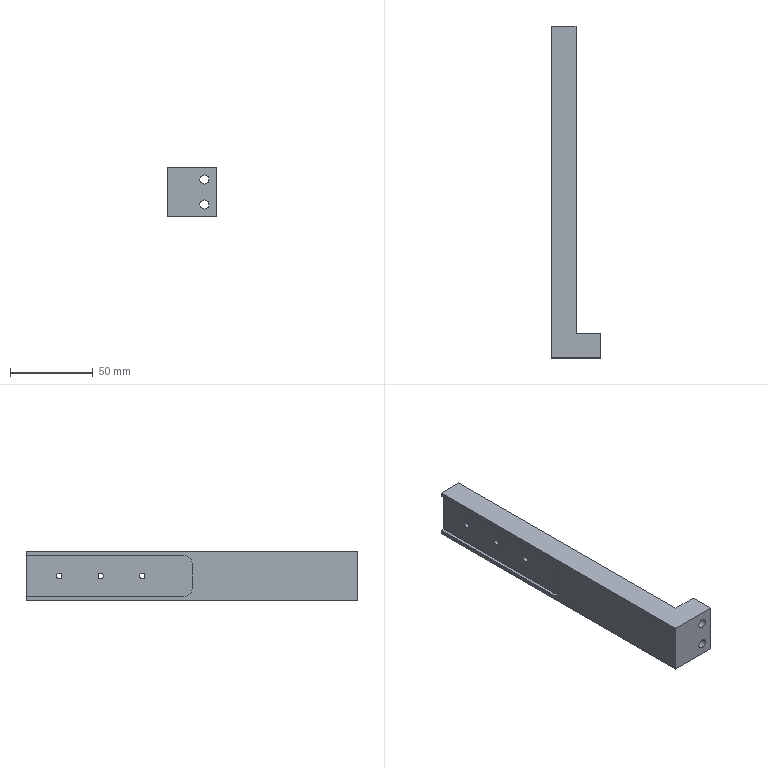Part | NX | 1 solid | 19 faces | box 30 x 200 x 30 mm | volume 90725 mm3 | plane 12 | cylinder 7 | commonest cylinder face diameters 3.3 x3 5.5 x2 10 x2
STEP:
#1=CARTESIAN_POINT('',(2.,105.,2.5));
#2=VERTEX_POINT('',#1);
#3=CARTESIAN_POINT('',(2.,100.,7.5));
#4=VERTEX_POINT('',#3);
#5=CARTESIAN_POINT('',(2.,105.,7.5));
#6=DIRECTION('',(-1.,0.,0.));
#7=DIRECTION('',(0.,1.,0.));
#8=AXIS2_PLACEMENT_3D('',#5,#6,#7);
#9=CIRCLE('',#8,5.);
#10=EDGE_CURVE('',#2,#4,#9,.T.);
#11=ORIENTED_EDGE('',*,*,#10,.F.);
#12=CARTESIAN_POINT('',(0.,105.,2.5));
#13=VERTEX_POINT('',#12);
#14=CARTESIAN_POINT('',(2.,105.,2.5));
#15=DIRECTION('',(1.,0.,0.));
#16=VECTOR('',#15,1000.);
#17=LINE('',#14,#16);
#18=EDGE_CURVE('',#13,#2,#17,.T.);
#19=ORIENTED_EDGE('',*,*,#18,.F.);
#20=CARTESIAN_POINT('',(0.,100.,7.5));
#21=VERTEX_POINT('',#20);
#22=CARTESIAN_POINT('',(0.,105.,7.5));
#23=DIRECTION('',(1.,0.,0.));
#24=DIRECTION('',(0.,1.,0.));
#25=AXIS2_PLACEMENT_3D('',#22,#23,#24);
#26=CIRCLE('',#25,5.);
#27=EDGE_CURVE('',#21,#13,#26,.T.);
#28=ORIENTED_EDGE('',*,*,#27,.F.);
#29=CARTESIAN_POINT('',(0.,100.,7.5));
#30=DIRECTION('',(-1.,0.,0.));
#31=VECTOR('',#30,1000.);
#32=LINE('',#29,#31);
#33=EDGE_CURVE('',#4,#21,#32,.T.);
#34=ORIENTED_EDGE('',*,*,#33,.F.);
#35=EDGE_LOOP('',(#11,#19,#28,#34));
#36=FACE_BOUND('',#35,.T.);
#37=CARTESIAN_POINT('',(2.,105.,7.5));
#38=DIRECTION('',(1.,0.,0.));
#39=DIRECTION('',(0.,1.,0.));
#40=AXIS2_PLACEMENT_3D('',#37,#38,#39);
#41=CYLINDRICAL_SURFACE('',#40,5.);
#42=ADVANCED_FACE('',(#36),#41,.F.);
#43=CARTESIAN_POINT('',(2.,100.,22.5));
#44=VERTEX_POINT('',#43);
#45=CARTESIAN_POINT('',(2.,105.,27.5));
#46=VERTEX_POINT('',#45);
#47=CARTESIAN_POINT('',(2.,105.,22.5));
#48=DIRECTION('',(-1.,0.,0.));
#49=DIRECTION('',(0.,1.,0.));
#50=AXIS2_PLACEMENT_3D('',#47,#48,#49);
#51=CIRCLE('',#50,5.);
#52=EDGE_CURVE('',#44,#46,#51,.T.);
#53=ORIENTED_EDGE('',*,*,#52,.F.);
#54=CARTESIAN_POINT('',(0.,100.,22.5));
#55=VERTEX_POINT('',#54);
#56=CARTESIAN_POINT('',(2.,100.,22.5));
#57=DIRECTION('',(1.,0.,0.));
#58=VECTOR('',#57,1000.);
#59=LINE('',#56,#58);
#60=EDGE_CURVE('',#55,#44,#59,.T.);
#61=ORIENTED_EDGE('',*,*,#60,.F.);
#62=CARTESIAN_POINT('',(0.,105.,27.5));
#63=VERTEX_POINT('',#62);
#64=CARTESIAN_POINT('',(0.,105.,22.5));
#65=DIRECTION('',(1.,0.,0.));
#66=DIRECTION('',(0.,1.,0.));
#67=AXIS2_PLACEMENT_3D('',#64,#65,#66);
#68=CIRCLE('',#67,5.);
#69=EDGE_CURVE('',#63,#55,#68,.T.);
#70=ORIENTED_EDGE('',*,*,#69,.F.);
#71=CARTESIAN_POINT('',(0.,105.,27.5));
#72=DIRECTION('',(-1.,0.,0.));
#73=VECTOR('',#72,1000.);
#74=LINE('',#71,#73);
#75=EDGE_CURVE('',#46,#63,#74,.T.);
#76=ORIENTED_EDGE('',*,*,#75,.F.);
#77=EDGE_LOOP('',(#53,#61,#70,#76));
#78=FACE_BOUND('',#77,.T.);
#79=CARTESIAN_POINT('',(2.,105.,22.5));
#80=DIRECTION('',(1.,0.,0.));
#81=DIRECTION('',(0.,1.,0.));
#82=AXIS2_PLACEMENT_3D('',#79,#80,#81);
#83=CYLINDRICAL_SURFACE('',#82,5.);
#84=ADVANCED_FACE('',(#78),#83,.F.);
#85=CARTESIAN_POINT('',(2.,100.,27.5));
#86=DIRECTION('',(0.,0.,1.));
#87=VECTOR('',#86,1000.);
#88=LINE('',#85,#87);
#89=EDGE_CURVE('',#4,#44,#88,.T.);
#90=ORIENTED_EDGE('',*,*,#89,.T.);
#91=ORIENTED_EDGE('',*,*,#52,.T.);
#92=CARTESIAN_POINT('',(2.,200.,27.5));
#93=VERTEX_POINT('',#92);
#94=CARTESIAN_POINT('',(2.,200.,27.5));
#95=DIRECTION('',(0.,1.,0.));
#96=VECTOR('',#95,1000.);
#97=LINE('',#94,#96);
#98=EDGE_CURVE('',#46,#93,#97,.T.);
#99=ORIENTED_EDGE('',*,*,#98,.T.);
#100=CARTESIAN_POINT('',(2.,200.,2.5));
#101=VERTEX_POINT('',#100);
#102=CARTESIAN_POINT('',(2.,200.,27.5));
#103=DIRECTION('',(0.,0.,-1.));
#104=VECTOR('',#103,1000.);
#105=LINE('',#102,#104);
#106=EDGE_CURVE('',#93,#101,#105,.T.);
#107=ORIENTED_EDGE('',*,*,#106,.T.);
#108=CARTESIAN_POINT('',(2.,200.,2.5));
#109=DIRECTION('',(0.,-1.,0.));
#110=VECTOR('',#109,1000.);
#111=LINE('',#108,#110);
#112=EDGE_CURVE('',#101,#2,#111,.T.);
#113=ORIENTED_EDGE('',*,*,#112,.T.);
#114=ORIENTED_EDGE('',*,*,#10,.T.);
#115=EDGE_LOOP('',(#90,#91,#99,#107,#113,#114));
#116=FACE_BOUND('',#115,.T.);
#117=CARTESIAN_POINT('',(2.,130.,16.65));
#118=VERTEX_POINT('',#117);
#119=CARTESIAN_POINT('',(2.,130.,15.));
#120=DIRECTION('',(-1.,0.,0.));
#121=DIRECTION('',(0.,0.,1.));
#122=AXIS2_PLACEMENT_3D('',#119,#120,#121);
#123=CIRCLE('',#122,1.65);
#124=EDGE_CURVE('',#118,#118,#123,.T.);
#125=ORIENTED_EDGE('',*,*,#124,.F.);
#126=EDGE_LOOP('',(#125));
#127=FACE_BOUND('',#126,.T.);
#128=CARTESIAN_POINT('',(2.,155.,16.65));
#129=VERTEX_POINT('',#128);
#130=CARTESIAN_POINT('',(2.,155.,15.));
#131=DIRECTION('',(-1.,0.,0.));
#132=DIRECTION('',(0.,0.,1.));
#133=AXIS2_PLACEMENT_3D('',#130,#131,#132);
#134=CIRCLE('',#133,1.65);
#135=EDGE_CURVE('',#129,#129,#134,.T.);
#136=ORIENTED_EDGE('',*,*,#135,.F.);
#137=EDGE_LOOP('',(#136));
#138=FACE_BOUND('',#137,.T.);
#139=CARTESIAN_POINT('',(2.,180.,16.65));
#140=VERTEX_POINT('',#139);
#141=CARTESIAN_POINT('',(2.,180.,15.));
#142=DIRECTION('',(-1.,0.,0.));
#143=DIRECTION('',(0.,0.,1.));
#144=AXIS2_PLACEMENT_3D('',#141,#142,#143);
#145=CIRCLE('',#144,1.65);
#146=EDGE_CURVE('',#140,#140,#145,.T.);
#147=ORIENTED_EDGE('',*,*,#146,.F.);
#148=EDGE_LOOP('',(#147));
#149=FACE_BOUND('',#148,.T.);
#150=CARTESIAN_POINT('',(2.,0.,0.));
#151=DIRECTION('',(1.,0.,0.));
#152=DIRECTION('',(0.,1.,0.));
#153=AXIS2_PLACEMENT_3D('',#150,#151,#152);
#154=PLANE('',#153);
#155=ADVANCED_FACE('',(#116,#127,#138,#149),#154,.F.);
#156=CARTESIAN_POINT('',(0.,200.,2.5));
#157=VERTEX_POINT('',#156);
#158=CARTESIAN_POINT('',(0.,200.,2.5));
#159=DIRECTION('',(0.,-1.,0.));
#160=VECTOR('',#159,1000.);
#161=LINE('',#158,#160);
#162=EDGE_CURVE('',#157,#13,#161,.T.);
#163=ORIENTED_EDGE('',*,*,#162,.T.);
#164=ORIENTED_EDGE('',*,*,#18,.T.);
#165=ORIENTED_EDGE('',*,*,#112,.F.);
#166=CARTESIAN_POINT('',(2.,200.,2.5));
#167=DIRECTION('',(-1.,0.,0.));
#168=VECTOR('',#167,1000.);
#169=LINE('',#166,#168);
#170=EDGE_CURVE('',#101,#157,#169,.T.);
#171=ORIENTED_EDGE('',*,*,#170,.T.);
#172=EDGE_LOOP('',(#163,#164,#165,#171));
#173=FACE_BOUND('',#172,.T.);
#174=CARTESIAN_POINT('',(2.,200.,2.5));
#175=DIRECTION('',(0.,0.,-1.));
#176=DIRECTION('',(0.,1.,0.));
#177=AXIS2_PLACEMENT_3D('',#174,#175,#176);
#178=PLANE('',#177);
#179=ADVANCED_FACE('',(#173),#178,.F.);
#180=CARTESIAN_POINT('',(0.,100.,27.5));
#181=DIRECTION('',(0.,0.,1.));
#182=VECTOR('',#181,1000.);
#183=LINE('',#180,#182);
#184=EDGE_CURVE('',#21,#55,#183,.T.);
#185=ORIENTED_EDGE('',*,*,#184,.T.);
#186=ORIENTED_EDGE('',*,*,#60,.T.);
#187=ORIENTED_EDGE('',*,*,#89,.F.);
#188=ORIENTED_EDGE('',*,*,#33,.T.);
#189=EDGE_LOOP('',(#185,#186,#187,#188));
#190=FACE_BOUND('',#189,.T.);
#191=CARTESIAN_POINT('',(2.,100.,27.5));
#192=DIRECTION('',(0.,-1.,0.));
#193=DIRECTION('',(1.,0.,0.));
#194=AXIS2_PLACEMENT_3D('',#191,#192,#193);
#195=PLANE('',#194);
#196=ADVANCED_FACE('',(#190),#195,.F.);
#197=ORIENTED_EDGE('',*,*,#98,.F.);
#198=ORIENTED_EDGE('',*,*,#75,.T.);
#199=CARTESIAN_POINT('',(0.,200.,27.5));
#200=VERTEX_POINT('',#199);
#201=CARTESIAN_POINT('',(0.,200.,27.5));
#202=DIRECTION('',(0.,1.,0.));
#203=VECTOR('',#202,1000.);
#204=LINE('',#201,#203);
#205=EDGE_CURVE('',#63,#200,#204,.T.);
#206=ORIENTED_EDGE('',*,*,#205,.T.);
#207=CARTESIAN_POINT('',(2.,200.,27.5));
#208=DIRECTION('',(-1.,0.,0.));
#209=VECTOR('',#208,1000.);
#210=LINE('',#207,#209);
#211=EDGE_CURVE('',#93,#200,#210,.T.);
#212=ORIENTED_EDGE('',*,*,#211,.F.);
#213=EDGE_LOOP('',(#197,#198,#206,#212));
#214=FACE_BOUND('',#213,.T.);
#215=CARTESIAN_POINT('',(2.,200.,27.5));
#216=DIRECTION('',(0.,0.,1.));
#217=DIRECTION('',(0.,-1.,0.));
#218=AXIS2_PLACEMENT_3D('',#215,#216,#217);
#219=PLANE('',#218);
#220=ADVANCED_FACE('',(#214),#219,.F.);
#221=CARTESIAN_POINT('',(0.,200.,0.));
#222=VERTEX_POINT('',#221);
#223=CARTESIAN_POINT('',(0.,0.,0.));
#224=VERTEX_POINT('',#223);
#225=CARTESIAN_POINT('',(0.,200.,0.));
#226=DIRECTION('',(0.,-1.,0.));
#227=VECTOR('',#226,1000.);
#228=LINE('',#225,#227);
#229=EDGE_CURVE('',#222,#224,#228,.T.);
#230=ORIENTED_EDGE('',*,*,#229,.F.);
#231=CARTESIAN_POINT('',(15.,200.,0.));
#232=VERTEX_POINT('',#231);
#233=CARTESIAN_POINT('',(15.,200.,0.));
#234=DIRECTION('',(-1.,0.,0.));
#235=VECTOR('',#234,1000.);
#236=LINE('',#233,#235);
#237=EDGE_CURVE('',#232,#222,#236,.T.);
#238=ORIENTED_EDGE('',*,*,#237,.F.);
#239=CARTESIAN_POINT('',(15.,15.,0.));
#240=VERTEX_POINT('',#239);
#241=CARTESIAN_POINT('',(15.,15.,0.));
#242=DIRECTION('',(0.,1.,0.));
#243=VECTOR('',#242,1000.);
#244=LINE('',#241,#243);
#245=EDGE_CURVE('',#240,#232,#244,.T.);
#246=ORIENTED_EDGE('',*,*,#245,.F.);
#247=CARTESIAN_POINT('',(30.,15.,0.));
#248=VERTEX_POINT('',#247);
#249=CARTESIAN_POINT('',(30.,15.,0.));
#250=DIRECTION('',(-1.,0.,0.));
#251=VECTOR('',#250,1000.);
#252=LINE('',#249,#251);
#253=EDGE_CURVE('',#248,#240,#252,.T.);
#254=ORIENTED_EDGE('',*,*,#253,.F.);
#255=CARTESIAN_POINT('',(30.,0.,0.));
#256=VERTEX_POINT('',#255);
#257=CARTESIAN_POINT('',(30.,0.,0.));
#258=DIRECTION('',(0.,1.,0.));
#259=VECTOR('',#258,1000.);
#260=LINE('',#257,#259);
#261=EDGE_CURVE('',#256,#248,#260,.T.);
#262=ORIENTED_EDGE('',*,*,#261,.F.);
#263=CARTESIAN_POINT('',(0.,0.,0.));
#264=DIRECTION('',(1.,0.,0.));
#265=VECTOR('',#264,1000.);
#266=LINE('',#263,#265);
#267=EDGE_CURVE('',#224,#256,#266,.T.);
#268=ORIENTED_EDGE('',*,*,#267,.F.);
#269=EDGE_LOOP('',(#230,#238,#246,#254,#262,#268));
#270=FACE_BOUND('',#269,.T.);
#271=CARTESIAN_POINT('',(0.,0.,0.));
#272=DIRECTION('',(0.,0.,1.));
#273=DIRECTION('',(1.,0.,0.));
#274=AXIS2_PLACEMENT_3D('',#271,#272,#273);
#275=PLANE('',#274);
#276=ADVANCED_FACE('',(#270),#275,.F.);
#277=CARTESIAN_POINT('',(0.,200.,30.));
#278=VERTEX_POINT('',#277);
#279=CARTESIAN_POINT('',(0.,0.,30.));
#280=VERTEX_POINT('',#279);
#281=CARTESIAN_POINT('',(0.,200.,30.));
#282=DIRECTION('',(0.,-1.,0.));
#283=VECTOR('',#282,1000.);
#284=LINE('',#281,#283);
#285=EDGE_CURVE('',#278,#280,#284,.T.);
#286=ORIENTED_EDGE('',*,*,#285,.T.);
#287=CARTESIAN_POINT('',(30.,0.,30.));
#288=VERTEX_POINT('',#287);
#289=CARTESIAN_POINT('',(0.,0.,30.));
#290=DIRECTION('',(1.,0.,0.));
#291=VECTOR('',#290,1000.);
#292=LINE('',#289,#291);
#293=EDGE_CURVE('',#280,#288,#292,.T.);
#294=ORIENTED_EDGE('',*,*,#293,.T.);
#295=CARTESIAN_POINT('',(30.,15.,30.));
#296=VERTEX_POINT('',#295);
#297=CARTESIAN_POINT('',(30.,0.,30.));
#298=DIRECTION('',(0.,1.,0.));
#299=VECTOR('',#298,1000.);
#300=LINE('',#297,#299);
#301=EDGE_CURVE('',#288,#296,#300,.T.);
#302=ORIENTED_EDGE('',*,*,#301,.T.);
#303=CARTESIAN_POINT('',(15.,15.,30.));
#304=VERTEX_POINT('',#303);
#305=CARTESIAN_POINT('',(30.,15.,30.));
#306=DIRECTION('',(-1.,0.,0.));
#307=VECTOR('',#306,1000.);
#308=LINE('',#305,#307);
#309=EDGE_CURVE('',#296,#304,#308,.T.);
#310=ORIENTED_EDGE('',*,*,#309,.T.);
#311=CARTESIAN_POINT('',(15.,200.,30.));
#312=VERTEX_POINT('',#311);
#313=CARTESIAN_POINT('',(15.,15.,30.));
#314=DIRECTION('',(0.,1.,0.));
#315=VECTOR('',#314,1000.);
#316=LINE('',#313,#315);
#317=EDGE_CURVE('',#304,#312,#316,.T.);
#318=ORIENTED_EDGE('',*,*,#317,.T.);
#319=CARTESIAN_POINT('',(15.,200.,30.));
#320=DIRECTION('',(-1.,0.,0.));
#321=VECTOR('',#320,1000.);
#322=LINE('',#319,#321);
#323=EDGE_CURVE('',#312,#278,#322,.T.);
#324=ORIENTED_EDGE('',*,*,#323,.T.);
#325=EDGE_LOOP('',(#286,#294,#302,#310,#318,#324));
#326=FACE_BOUND('',#325,.T.);
#327=CARTESIAN_POINT('',(0.,0.,30.));
#328=DIRECTION('',(0.,0.,1.));
#329=DIRECTION('',(1.,0.,0.));
#330=AXIS2_PLACEMENT_3D('',#327,#328,#329);
#331=PLANE('',#330);
#332=ADVANCED_FACE('',(#326),#331,.T.);
#333=ORIENTED_EDGE('',*,*,#106,.F.);
#334=ORIENTED_EDGE('',*,*,#211,.T.);
#335=CARTESIAN_POINT('',(0.,200.,30.));
#336=DIRECTION('',(0.,0.,-1.));
#337=VECTOR('',#336,1000.);
#338=LINE('',#335,#337);
#339=EDGE_CURVE('',#278,#200,#338,.T.);
#340=ORIENTED_EDGE('',*,*,#339,.F.);
#341=ORIENTED_EDGE('',*,*,#323,.F.);
#342=CARTESIAN_POINT('',(15.,200.,30.));
#343=DIRECTION('',(0.,0.,-1.));
#344=VECTOR('',#343,1000.);
#345=LINE('',#342,#344);
#346=EDGE_CURVE('',#312,#232,#345,.T.);
#347=ORIENTED_EDGE('',*,*,#346,.T.);
#348=ORIENTED_EDGE('',*,*,#237,.T.);
#349=CARTESIAN_POINT('',(0.,200.,30.));
#350=DIRECTION('',(0.,0.,-1.));
#351=VECTOR('',#350,1000.);
#352=LINE('',#349,#351);
#353=EDGE_CURVE('',#157,#222,#352,.T.);
#354=ORIENTED_EDGE('',*,*,#353,.F.);
#355=ORIENTED_EDGE('',*,*,#170,.F.);
#356=EDGE_LOOP('',(#333,#334,#340,#341,#347,#348,#354,#355));
#357=FACE_BOUND('',#356,.T.);
#358=CARTESIAN_POINT('',(15.,200.,30.));
#359=DIRECTION('',(0.,-1.,0.));
#360=DIRECTION('',(0.,0.,-1.));
#361=AXIS2_PLACEMENT_3D('',#358,#359,#360);
#362=PLANE('',#361);
#363=ADVANCED_FACE('',(#357),#362,.F.);
#364=ORIENTED_EDGE('',*,*,#245,.T.);
#365=ORIENTED_EDGE('',*,*,#346,.F.);
#366=ORIENTED_EDGE('',*,*,#317,.F.);
#367=CARTESIAN_POINT('',(15.,15.,30.));
#368=DIRECTION('',(0.,0.,-1.));
#369=VECTOR('',#368,1000.);
#370=LINE('',#367,#369);
#371=EDGE_CURVE('',#304,#240,#370,.T.);
#372=ORIENTED_EDGE('',*,*,#371,.T.);
#373=EDGE_LOOP('',(#364,#365,#366,#372));
#374=FACE_BOUND('',#373,.T.);
#375=CARTESIAN_POINT('',(15.,128.35,15.));
#376=VERTEX_POINT('',#375);
#377=CARTESIAN_POINT('',(15.,130.,15.));
#378=DIRECTION('',(-1.,0.,0.));
#379=DIRECTION('',(0.,-1.,0.));
#380=AXIS2_PLACEMENT_3D('',#377,#378,#379);
#381=CIRCLE('',#380,1.65);
#382=EDGE_CURVE('',#376,#376,#381,.T.);
#383=ORIENTED_EDGE('',*,*,#382,.T.);
#384=EDGE_LOOP('',(#383));
#385=FACE_BOUND('',#384,.T.);
#386=CARTESIAN_POINT('',(15.,153.35,15.));
#387=VERTEX_POINT('',#386);
#388=CARTESIAN_POINT('',(15.,155.,15.));
#389=DIRECTION('',(-1.,0.,0.));
#390=DIRECTION('',(0.,-1.,0.));
#391=AXIS2_PLACEMENT_3D('',#388,#389,#390);
#392=CIRCLE('',#391,1.65);
#393=EDGE_CURVE('',#387,#387,#392,.T.);
#394=ORIENTED_EDGE('',*,*,#393,.T.);
#395=EDGE_LOOP('',(#394));
#396=FACE_BOUND('',#395,.T.);
#397=CARTESIAN_POINT('',(15.,178.35,15.));
#398=VERTEX_POINT('',#397);
#399=CARTESIAN_POINT('',(15.,180.,15.));
#400=DIRECTION('',(-1.,0.,0.));
#401=DIRECTION('',(0.,-1.,0.));
#402=AXIS2_PLACEMENT_3D('',#399,#400,#401);
#403=CIRCLE('',#402,1.65);
#404=EDGE_CURVE('',#398,#398,#403,.T.);
#405=ORIENTED_EDGE('',*,*,#404,.T.);
#406=EDGE_LOOP('',(#405));
#407=FACE_BOUND('',#406,.T.);
#408=CARTESIAN_POINT('',(15.,15.,30.));
#409=DIRECTION('',(-1.,0.,0.));
#410=DIRECTION('',(0.,-1.,0.));
#411=AXIS2_PLACEMENT_3D('',#408,#409,#410);
#412=PLANE('',#411);
#413=ADVANCED_FACE('',(#374,#385,#396,#407),#412,.F.);
#414=ORIENTED_EDGE('',*,*,#253,.T.);
#415=ORIENTED_EDGE('',*,*,#371,.F.);
#416=ORIENTED_EDGE('',*,*,#309,.F.);
#417=CARTESIAN_POINT('',(30.,15.,30.));
#418=DIRECTION('',(0.,0.,-1.));
#419=VECTOR('',#418,1000.);
#420=LINE('',#417,#419);
#421=EDGE_CURVE('',#296,#248,#420,.T.);
#422=ORIENTED_EDGE('',*,*,#421,.T.);
#423=EDGE_LOOP('',(#414,#415,#416,#422));
#424=FACE_BOUND('',#423,.T.);
#425=CARTESIAN_POINT('',(22.5,15.,10.25));
#426=VERTEX_POINT('',#425);
#427=CARTESIAN_POINT('',(22.5,15.,7.5));
#428=DIRECTION('',(0.,1.,0.));
#429=DIRECTION('',(0.,0.,1.));
#430=AXIS2_PLACEMENT_3D('',#427,#428,#429);
#431=CIRCLE('',#430,2.75);
#432=EDGE_CURVE('',#426,#426,#431,.T.);
#433=ORIENTED_EDGE('',*,*,#432,.F.);
#434=EDGE_LOOP('',(#433));
#435=FACE_BOUND('',#434,.T.);
#436=CARTESIAN_POINT('',(22.5,15.,25.25));
#437=VERTEX_POINT('',#436);
#438=CARTESIAN_POINT('',(22.5,15.,22.5));
#439=DIRECTION('',(0.,1.,0.));
#440=DIRECTION('',(0.,0.,1.));
#441=AXIS2_PLACEMENT_3D('',#438,#439,#440);
#442=CIRCLE('',#441,2.75);
#443=EDGE_CURVE('',#437,#437,#442,.T.);
#444=ORIENTED_EDGE('',*,*,#443,.F.);
#445=EDGE_LOOP('',(#444));
#446=FACE_BOUND('',#445,.T.);
#447=CARTESIAN_POINT('',(30.,15.,30.));
#448=DIRECTION('',(0.,-1.,0.));
#449=DIRECTION('',(1.,0.,0.));
#450=AXIS2_PLACEMENT_3D('',#447,#448,#449);
#451=PLANE('',#450);
#452=ADVANCED_FACE('',(#424,#435,#446),#451,.F.);
#453=ORIENTED_EDGE('',*,*,#261,.T.);
#454=ORIENTED_EDGE('',*,*,#421,.F.);
#455=ORIENTED_EDGE('',*,*,#301,.F.);
#456=CARTESIAN_POINT('',(30.,0.,30.));
#457=DIRECTION('',(0.,0.,-1.));
#458=VECTOR('',#457,1000.);
#459=LINE('',#456,#458);
#460=EDGE_CURVE('',#288,#256,#459,.T.);
#461=ORIENTED_EDGE('',*,*,#460,.T.);
#462=EDGE_LOOP('',(#453,#454,#455,#461));
#463=FACE_BOUND('',#462,.T.);
#464=CARTESIAN_POINT('',(30.,0.,30.));
#465=DIRECTION('',(-1.,0.,0.));
#466=DIRECTION('',(0.,0.,1.));
#467=AXIS2_PLACEMENT_3D('',#464,#465,#466);
#468=PLANE('',#467);
#469=ADVANCED_FACE('',(#463),#468,.F.);
#470=ORIENTED_EDGE('',*,*,#267,.T.);
#471=ORIENTED_EDGE('',*,*,#460,.F.);
#472=ORIENTED_EDGE('',*,*,#293,.F.);
#473=CARTESIAN_POINT('',(0.,0.,30.));
#474=DIRECTION('',(0.,0.,-1.));
#475=VECTOR('',#474,1000.);
#476=LINE('',#473,#475);
#477=EDGE_CURVE('',#280,#224,#476,.T.);
#478=ORIENTED_EDGE('',*,*,#477,.T.);
#479=EDGE_LOOP('',(#470,#471,#472,#478));
#480=FACE_BOUND('',#479,.T.);
#481=CARTESIAN_POINT('',(22.5,0.,10.25));
#482=VERTEX_POINT('',#481);
#483=CARTESIAN_POINT('',(22.5,0.,7.5));
#484=DIRECTION('',(0.,1.,0.));
#485=DIRECTION('',(0.,0.,1.));
#486=AXIS2_PLACEMENT_3D('',#483,#484,#485);
#487=CIRCLE('',#486,2.75);
#488=EDGE_CURVE('',#482,#482,#487,.T.);
#489=ORIENTED_EDGE('',*,*,#488,.T.);
#490=EDGE_LOOP('',(#489));
#491=FACE_BOUND('',#490,.T.);
#492=CARTESIAN_POINT('',(22.5,0.,25.25));
#493=VERTEX_POINT('',#492);
#494=CARTESIAN_POINT('',(22.5,0.,22.5));
#495=DIRECTION('',(0.,1.,0.));
#496=DIRECTION('',(0.,0.,1.));
#497=AXIS2_PLACEMENT_3D('',#494,#495,#496);
#498=CIRCLE('',#497,2.75);
#499=EDGE_CURVE('',#493,#493,#498,.T.);
#500=ORIENTED_EDGE('',*,*,#499,.T.);
#501=EDGE_LOOP('',(#500));
#502=FACE_BOUND('',#501,.T.);
#503=CARTESIAN_POINT('',(0.,0.,30.));
#504=DIRECTION('',(0.,1.,0.));
#505=DIRECTION('',(0.,0.,1.));
#506=AXIS2_PLACEMENT_3D('',#503,#504,#505);
#507=PLANE('',#506);
#508=ADVANCED_FACE('',(#480,#491,#502),#507,.F.);
#509=ORIENTED_EDGE('',*,*,#339,.T.);
#510=ORIENTED_EDGE('',*,*,#205,.F.);
#511=ORIENTED_EDGE('',*,*,#69,.T.);
#512=ORIENTED_EDGE('',*,*,#184,.F.);
#513=ORIENTED_EDGE('',*,*,#27,.T.);
#514=ORIENTED_EDGE('',*,*,#162,.F.);
#515=ORIENTED_EDGE('',*,*,#353,.T.);
#516=ORIENTED_EDGE('',*,*,#229,.T.);
#517=ORIENTED_EDGE('',*,*,#477,.F.);
#518=ORIENTED_EDGE('',*,*,#285,.F.);
#519=EDGE_LOOP('',(#509,#510,#511,#512,#513,#514,#515,#516,#517,#518));
#520=FACE_BOUND('',#519,.T.);
#521=CARTESIAN_POINT('',(0.,200.,30.));
#522=DIRECTION('',(1.,0.,0.));
#523=DIRECTION('',(0.,1.,0.));
#524=AXIS2_PLACEMENT_3D('',#521,#522,#523);
#525=PLANE('',#524);
#526=ADVANCED_FACE('',(#520),#525,.F.);
#527=ORIENTED_EDGE('',*,*,#488,.F.);
#528=EDGE_LOOP('',(#527));
#529=FACE_BOUND('',#528,.T.);
#530=ORIENTED_EDGE('',*,*,#432,.T.);
#531=EDGE_LOOP('',(#530));
#532=FACE_BOUND('',#531,.T.);
#533=CARTESIAN_POINT('',(22.5,15.,7.5));
#534=DIRECTION('',(0.,1.,0.));
#535=DIRECTION('',(0.,0.,1.));
#536=AXIS2_PLACEMENT_3D('',#533,#534,#535);
#537=CYLINDRICAL_SURFACE('',#536,2.75);
#538=ADVANCED_FACE('',(#529,#532),#537,.F.);
#539=ORIENTED_EDGE('',*,*,#499,.F.);
#540=EDGE_LOOP('',(#539));
#541=FACE_BOUND('',#540,.T.);
#542=ORIENTED_EDGE('',*,*,#443,.T.);
#543=EDGE_LOOP('',(#542));
#544=FACE_BOUND('',#543,.T.);
#545=CARTESIAN_POINT('',(22.5,15.,22.5));
#546=DIRECTION('',(0.,1.,0.));
#547=DIRECTION('',(0.,0.,1.));
#548=AXIS2_PLACEMENT_3D('',#545,#546,#547);
#549=CYLINDRICAL_SURFACE('',#548,2.75);
#550=ADVANCED_FACE('',(#541,#544),#549,.F.);
#551=ORIENTED_EDGE('',*,*,#382,.F.);
#552=EDGE_LOOP('',(#551));
#553=FACE_BOUND('',#552,.T.);
#554=ORIENTED_EDGE('',*,*,#124,.T.);
#555=EDGE_LOOP('',(#554));
#556=FACE_BOUND('',#555,.T.);
#557=CARTESIAN_POINT('',(2.,130.,15.));
#558=DIRECTION('',(-1.,0.,0.));
#559=DIRECTION('',(0.,0.,1.));
#560=AXIS2_PLACEMENT_3D('',#557,#558,#559);
#561=CYLINDRICAL_SURFACE('',#560,1.65);
#562=ADVANCED_FACE('',(#553,#556),#561,.F.);
#563=ORIENTED_EDGE('',*,*,#393,.F.);
#564=EDGE_LOOP('',(#563));
#565=FACE_BOUND('',#564,.T.);
#566=ORIENTED_EDGE('',*,*,#135,.T.);
#567=EDGE_LOOP('',(#566));
#568=FACE_BOUND('',#567,.T.);
#569=CARTESIAN_POINT('',(2.,155.,15.));
#570=DIRECTION('',(-1.,0.,0.));
#571=DIRECTION('',(0.,0.,1.));
#572=AXIS2_PLACEMENT_3D('',#569,#570,#571);
#573=CYLINDRICAL_SURFACE('',#572,1.65);
#574=ADVANCED_FACE('',(#565,#568),#573,.F.);
#575=ORIENTED_EDGE('',*,*,#404,.F.);
#576=EDGE_LOOP('',(#575));
#577=FACE_BOUND('',#576,.T.);
#578=ORIENTED_EDGE('',*,*,#146,.T.);
#579=EDGE_LOOP('',(#578));
#580=FACE_BOUND('',#579,.T.);
#581=CARTESIAN_POINT('',(2.,180.,15.));
#582=DIRECTION('',(-1.,0.,0.));
#583=DIRECTION('',(0.,0.,1.));
#584=AXIS2_PLACEMENT_3D('',#581,#582,#583);
#585=CYLINDRICAL_SURFACE('',#584,1.65);
#586=ADVANCED_FACE('',(#577,#580),#585,.F.);
#587=CLOSED_SHELL('',(#42,#84,#155,#179,#196,#220,#276,#332,#363,#413,#452,#469,#508,#526,#538,#550,#562,#574,#586));
#588=MANIFOLD_SOLID_BREP('',#587);
#589=(LENGTH_UNIT()NAMED_UNIT(*)SI_UNIT(.MILLI.,.METRE.));
#590=UNCERTAINTY_MEASURE_WITH_UNIT(LENGTH_MEASURE(0.00001),#589,'','');
#591=(NAMED_UNIT(*)PLANE_ANGLE_UNIT()SI_UNIT($,.RADIAN.));
#592=(NAMED_UNIT(*)SI_UNIT($,.STERADIAN.)SOLID_ANGLE_UNIT());
#593=(GEOMETRIC_REPRESENTATION_CONTEXT(3)GLOBAL_UNCERTAINTY_ASSIGNED_CONTEXT((#590))GLOBAL_UNIT_ASSIGNED_CONTEXT((#589,#591,#592))REPRESENTATION_CONTEXT('',''));
#594=ADVANCED_BREP_SHAPE_REPRESENTATION('',(#588),#593);